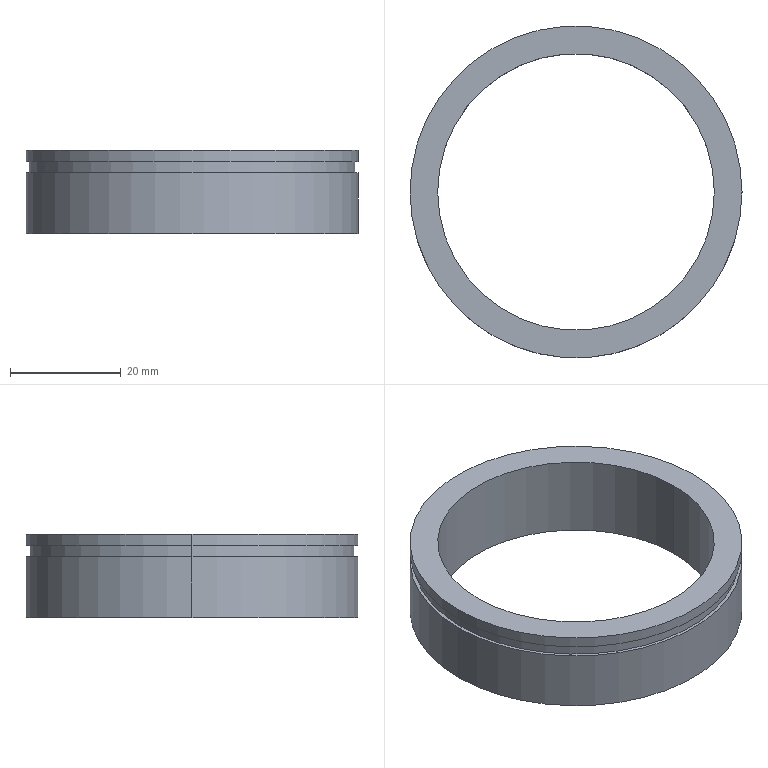Part | STEP file | 1 solid | 12 faces | box 60 x 60 x 15 mm | volume 12735 mm3 | cylinder 8 | plane 4 | commonest cylinder face diameters 60 x4 50 x2 58.8 x2
STEP:
#1=CARTESIAN_POINT('',(0.,0.,0.));
#2=DIRECTION('',(0.,0.,1.));
#3=DIRECTION('',(1.,0.,0.));
#4=AXIS2_PLACEMENT_3D('',#1,#2,#3);
#5=CARTESIAN_POINT('',(29.4,0.,11.));
#6=VERTEX_POINT('',#5);
#7=CARTESIAN_POINT('',(-29.4,0.,11.));
#8=VERTEX_POINT('',#7);
#9=CARTESIAN_POINT('',(0.,0.,11.));
#10=DIRECTION('',(0.,0.,1.));
#11=DIRECTION('',(1.,0.,0.));
#12=AXIS2_PLACEMENT_3D('',#9,#10,#11);
#13=CIRCLE('',#12,29.4);
#14=CARTESIAN_POINT('',(0.,0.,11.));
#15=DIRECTION('',(0.,0.,1.));
#16=DIRECTION('',(1.,0.,0.));
#17=AXIS2_PLACEMENT_3D('',#14,#15,#16);
#18=CYLINDRICAL_SURFACE('',#17,29.4);
#19=CARTESIAN_POINT('',(0.,0.));
#20=DIRECTION('',(1.,0.));
#21=VECTOR('',#20,1.);
#22=LINE('',#19,#21);
#23=(GEOMETRIC_REPRESENTATION_CONTEXT(2)PARAMETRIC_REPRESENTATION_CONTEXT()REPRESENTATION_CONTEXT('',''));
#24=DEFINITIONAL_REPRESENTATION('',(#22),#23);
#25=PCURVE('',#18,#24);
#26=CARTESIAN_POINT('',(0.,0.,11.));
#27=DIRECTION('',(0.,0.,1.));
#28=DIRECTION('',(1.,0.,0.));
#29=AXIS2_PLACEMENT_3D('',#26,#27,#28);
#30=PLANE('',#29);
#31=CARTESIAN_POINT('',(0.,0.));
#32=DIRECTION('',(1.,0.));
#33=AXIS2_PLACEMENT_2D('',#31,#32);
#34=CIRCLE('',#33,29.4);
#35=(GEOMETRIC_REPRESENTATION_CONTEXT(2)PARAMETRIC_REPRESENTATION_CONTEXT()REPRESENTATION_CONTEXT('',''));
#36=DEFINITIONAL_REPRESENTATION('',(#34),#35);
#37=PCURVE('',#30,#36);
#38=SURFACE_CURVE('',#13,(#25,#37),.PCURVE_S1.);
#39=EDGE_CURVE('',#6,#8,#38,.T.);
#40=ORIENTED_EDGE('',*,*,#39,.T.);
#41=CARTESIAN_POINT('',(-29.4,0.,13.));
#42=VERTEX_POINT('',#41);
#43=CARTESIAN_POINT('',(-29.4,0.,11.));
#44=DIRECTION('',(0.,0.,1.));
#45=VECTOR('',#44,1.);
#46=LINE('',#43,#45);
#47=CARTESIAN_POINT('',(3.142,0.));
#48=DIRECTION('',(0.,1.));
#49=VECTOR('',#48,1.);
#50=LINE('',#47,#49);
#51=(GEOMETRIC_REPRESENTATION_CONTEXT(2)PARAMETRIC_REPRESENTATION_CONTEXT()REPRESENTATION_CONTEXT('',''));
#52=DEFINITIONAL_REPRESENTATION('',(#50),#51);
#53=PCURVE('',#18,#52);
#54=CARTESIAN_POINT('',(0.,0.,11.));
#55=DIRECTION('',(0.,0.,1.));
#56=DIRECTION('',(1.,0.,0.));
#57=AXIS2_PLACEMENT_3D('',#54,#55,#56);
#58=CYLINDRICAL_SURFACE('',#57,29.4);
#59=CARTESIAN_POINT('',(3.142,0.));
#60=DIRECTION('',(0.,1.));
#61=VECTOR('',#60,1.);
#62=LINE('',#59,#61);
#63=(GEOMETRIC_REPRESENTATION_CONTEXT(2)PARAMETRIC_REPRESENTATION_CONTEXT()REPRESENTATION_CONTEXT('',''));
#64=DEFINITIONAL_REPRESENTATION('',(#62),#63);
#65=PCURVE('',#58,#64);
#66=SURFACE_CURVE('',#46,(#53,#65),.PCURVE_S1.);
#67=EDGE_CURVE('',#8,#42,#66,.T.);
#68=ORIENTED_EDGE('',*,*,#67,.T.);
#69=CARTESIAN_POINT('',(29.4,0.,13.));
#70=VERTEX_POINT('',#69);
#71=CARTESIAN_POINT('',(0.,0.,13.));
#72=DIRECTION('',(0.,0.,1.));
#73=DIRECTION('',(1.,0.,0.));
#74=AXIS2_PLACEMENT_3D('',#71,#72,#73);
#75=CIRCLE('',#74,29.4);
#76=CARTESIAN_POINT('',(0.,2.));
#77=DIRECTION('',(1.,0.));
#78=VECTOR('',#77,1.);
#79=LINE('',#76,#78);
#80=(GEOMETRIC_REPRESENTATION_CONTEXT(2)PARAMETRIC_REPRESENTATION_CONTEXT()REPRESENTATION_CONTEXT('',''));
#81=DEFINITIONAL_REPRESENTATION('',(#79),#80);
#82=PCURVE('',#18,#81);
#83=CARTESIAN_POINT('',(0.,0.,13.));
#84=DIRECTION('',(0.,0.,1.));
#85=DIRECTION('',(1.,0.,0.));
#86=AXIS2_PLACEMENT_3D('',#83,#84,#85);
#87=PLANE('',#86);
#88=CARTESIAN_POINT('',(0.,0.));
#89=DIRECTION('',(1.,0.));
#90=AXIS2_PLACEMENT_2D('',#88,#89);
#91=CIRCLE('',#90,29.4);
#92=(GEOMETRIC_REPRESENTATION_CONTEXT(2)PARAMETRIC_REPRESENTATION_CONTEXT()REPRESENTATION_CONTEXT('',''));
#93=DEFINITIONAL_REPRESENTATION('',(#91),#92);
#94=PCURVE('',#87,#93);
#95=SURFACE_CURVE('',#75,(#82,#94),.PCURVE_S1.);
#96=EDGE_CURVE('',#70,#42,#95,.T.);
#97=ORIENTED_EDGE('',*,*,#96,.F.);
#98=CARTESIAN_POINT('',(29.4,0.,11.));
#99=DIRECTION('',(0.,0.,1.));
#100=VECTOR('',#99,1.);
#101=LINE('',#98,#100);
#102=CARTESIAN_POINT('',(0.,0.));
#103=DIRECTION('',(0.,1.));
#104=VECTOR('',#103,1.);
#105=LINE('',#102,#104);
#106=(GEOMETRIC_REPRESENTATION_CONTEXT(2)PARAMETRIC_REPRESENTATION_CONTEXT()REPRESENTATION_CONTEXT('',''));
#107=DEFINITIONAL_REPRESENTATION('',(#105),#106);
#108=PCURVE('',#18,#107);
#109=CARTESIAN_POINT('',(6.283,0.));
#110=DIRECTION('',(0.,1.));
#111=VECTOR('',#110,1.);
#112=LINE('',#109,#111);
#113=(GEOMETRIC_REPRESENTATION_CONTEXT(2)PARAMETRIC_REPRESENTATION_CONTEXT()REPRESENTATION_CONTEXT('',''));
#114=DEFINITIONAL_REPRESENTATION('',(#112),#113);
#115=PCURVE('',#58,#114);
#116=SURFACE_CURVE('',#101,(#108,#115),.PCURVE_S1.);
#117=EDGE_CURVE('',#6,#70,#116,.T.);
#118=ORIENTED_EDGE('',*,*,#117,.F.);
#119=EDGE_LOOP('',(#40,#68,#97,#118));
#120=FACE_BOUND('',#119,.T.);
#121=ADVANCED_FACE('',(#120),#18,.T.);
#122=CARTESIAN_POINT('',(-25.,0.,15.));
#123=VERTEX_POINT('',#122);
#124=CARTESIAN_POINT('',(-25.,0.,0.));
#125=VERTEX_POINT('',#124);
#126=CARTESIAN_POINT('',(-25.,0.,15.));
#127=DIRECTION('',(0.,0.,-1.));
#128=VECTOR('',#127,1.);
#129=LINE('',#126,#128);
#130=CARTESIAN_POINT('',(0.,0.,15.));
#131=DIRECTION('',(0.,0.,-1.));
#132=DIRECTION('',(-1.,0.,0.));
#133=AXIS2_PLACEMENT_3D('',#130,#131,#132);
#134=CYLINDRICAL_SURFACE('',#133,25.);
#135=CARTESIAN_POINT('',(6.283,0.));
#136=DIRECTION('',(0.,1.));
#137=VECTOR('',#136,1.);
#138=LINE('',#135,#137);
#139=(GEOMETRIC_REPRESENTATION_CONTEXT(2)PARAMETRIC_REPRESENTATION_CONTEXT()REPRESENTATION_CONTEXT('',''));
#140=DEFINITIONAL_REPRESENTATION('',(#138),#139);
#141=PCURVE('',#134,#140);
#142=CARTESIAN_POINT('',(0.,0.,15.));
#143=DIRECTION('',(0.,0.,-1.));
#144=DIRECTION('',(-1.,0.,0.));
#145=AXIS2_PLACEMENT_3D('',#142,#143,#144);
#146=CYLINDRICAL_SURFACE('',#145,25.);
#147=CARTESIAN_POINT('',(0.,0.));
#148=DIRECTION('',(0.,1.));
#149=VECTOR('',#148,1.);
#150=LINE('',#147,#149);
#151=(GEOMETRIC_REPRESENTATION_CONTEXT(2)PARAMETRIC_REPRESENTATION_CONTEXT()REPRESENTATION_CONTEXT('',''));
#152=DEFINITIONAL_REPRESENTATION('',(#150),#151);
#153=PCURVE('',#146,#152);
#154=SURFACE_CURVE('',#129,(#141,#153),.PCURVE_S1.);
#155=EDGE_CURVE('',#123,#125,#154,.T.);
#156=ORIENTED_EDGE('',*,*,#155,.T.);
#157=CARTESIAN_POINT('',(25.,0.,0.));
#158=VERTEX_POINT('',#157);
#159=CARTESIAN_POINT('',(0.,0.,0.));
#160=DIRECTION('',(0.,0.,1.));
#161=DIRECTION('',(1.,0.,0.));
#162=AXIS2_PLACEMENT_3D('',#159,#160,#161);
#163=CIRCLE('',#162,25.);
#164=CARTESIAN_POINT('',(9.425,15.));
#165=DIRECTION('',(-1.,0.));
#166=VECTOR('',#165,1.);
#167=LINE('',#164,#166);
#168=(GEOMETRIC_REPRESENTATION_CONTEXT(2)PARAMETRIC_REPRESENTATION_CONTEXT()REPRESENTATION_CONTEXT('',''));
#169=DEFINITIONAL_REPRESENTATION('',(#167),#168);
#170=PCURVE('',#134,#169);
#171=CARTESIAN_POINT('',(0.,0.,0.));
#172=DIRECTION('',(0.,0.,1.));
#173=DIRECTION('',(1.,0.,0.));
#174=AXIS2_PLACEMENT_3D('',#171,#172,#173);
#175=PLANE('',#174);
#176=CARTESIAN_POINT('',(0.,0.));
#177=DIRECTION('',(1.,0.));
#178=AXIS2_PLACEMENT_2D('',#176,#177);
#179=CIRCLE('',#178,25.);
#180=(GEOMETRIC_REPRESENTATION_CONTEXT(2)PARAMETRIC_REPRESENTATION_CONTEXT()REPRESENTATION_CONTEXT('',''));
#181=DEFINITIONAL_REPRESENTATION('',(#179),#180);
#182=PCURVE('',#175,#181);
#183=SURFACE_CURVE('',#163,(#170,#182),.PCURVE_S1.);
#184=EDGE_CURVE('',#125,#158,#183,.T.);
#185=ORIENTED_EDGE('',*,*,#184,.T.);
#186=CARTESIAN_POINT('',(25.,0.,15.));
#187=VERTEX_POINT('',#186);
#188=CARTESIAN_POINT('',(25.,0.,15.));
#189=DIRECTION('',(0.,0.,-1.));
#190=VECTOR('',#189,1.);
#191=LINE('',#188,#190);
#192=CARTESIAN_POINT('',(3.142,0.));
#193=DIRECTION('',(0.,1.));
#194=VECTOR('',#193,1.);
#195=LINE('',#192,#194);
#196=(GEOMETRIC_REPRESENTATION_CONTEXT(2)PARAMETRIC_REPRESENTATION_CONTEXT()REPRESENTATION_CONTEXT('',''));
#197=DEFINITIONAL_REPRESENTATION('',(#195),#196);
#198=PCURVE('',#134,#197);
#199=CARTESIAN_POINT('',(3.142,0.));
#200=DIRECTION('',(0.,1.));
#201=VECTOR('',#200,1.);
#202=LINE('',#199,#201);
#203=(GEOMETRIC_REPRESENTATION_CONTEXT(2)PARAMETRIC_REPRESENTATION_CONTEXT()REPRESENTATION_CONTEXT('',''));
#204=DEFINITIONAL_REPRESENTATION('',(#202),#203);
#205=PCURVE('',#146,#204);
#206=SURFACE_CURVE('',#191,(#198,#205),.PCURVE_S1.);
#207=EDGE_CURVE('',#187,#158,#206,.T.);
#208=ORIENTED_EDGE('',*,*,#207,.F.);
#209=CARTESIAN_POINT('',(0.,0.,15.));
#210=DIRECTION('',(0.,0.,1.));
#211=DIRECTION('',(1.,0.,0.));
#212=AXIS2_PLACEMENT_3D('',#209,#210,#211);
#213=CIRCLE('',#212,25.);
#214=CARTESIAN_POINT('',(9.425,0.));
#215=DIRECTION('',(-1.,0.));
#216=VECTOR('',#215,1.);
#217=LINE('',#214,#216);
#218=(GEOMETRIC_REPRESENTATION_CONTEXT(2)PARAMETRIC_REPRESENTATION_CONTEXT()REPRESENTATION_CONTEXT('',''));
#219=DEFINITIONAL_REPRESENTATION('',(#217),#218);
#220=PCURVE('',#134,#219);
#221=CARTESIAN_POINT('',(0.,0.,15.));
#222=DIRECTION('',(0.,0.,1.));
#223=DIRECTION('',(1.,0.,0.));
#224=AXIS2_PLACEMENT_3D('',#221,#222,#223);
#225=PLANE('',#224);
#226=CARTESIAN_POINT('',(0.,0.));
#227=DIRECTION('',(1.,0.));
#228=AXIS2_PLACEMENT_2D('',#226,#227);
#229=CIRCLE('',#228,25.);
#230=(GEOMETRIC_REPRESENTATION_CONTEXT(2)PARAMETRIC_REPRESENTATION_CONTEXT()REPRESENTATION_CONTEXT('',''));
#231=DEFINITIONAL_REPRESENTATION('',(#229),#230);
#232=PCURVE('',#225,#231);
#233=SURFACE_CURVE('',#213,(#220,#232),.PCURVE_S1.);
#234=EDGE_CURVE('',#123,#187,#233,.T.);
#235=ORIENTED_EDGE('',*,*,#234,.F.);
#236=EDGE_LOOP('',(#156,#185,#208,#235));
#237=FACE_BOUND('',#236,.F.);
#238=ADVANCED_FACE('',(#237),#134,.F.);
#239=CARTESIAN_POINT('',(30.,0.,15.));
#240=VERTEX_POINT('',#239);
#241=CARTESIAN_POINT('',(-30.,0.,15.));
#242=VERTEX_POINT('',#241);
#243=CARTESIAN_POINT('',(0.,0.,15.));
#244=DIRECTION('',(0.,0.,1.));
#245=DIRECTION('',(1.,0.,0.));
#246=AXIS2_PLACEMENT_3D('',#243,#244,#245);
#247=CIRCLE('',#246,30.);
#248=CARTESIAN_POINT('',(0.,0.,15.));
#249=DIRECTION('',(0.,0.,-1.));
#250=DIRECTION('',(-1.,0.,0.));
#251=AXIS2_PLACEMENT_3D('',#248,#249,#250);
#252=CYLINDRICAL_SURFACE('',#251,30.);
#253=CARTESIAN_POINT('',(3.142,0.));
#254=DIRECTION('',(-1.,0.));
#255=VECTOR('',#254,1.);
#256=LINE('',#253,#255);
#257=(GEOMETRIC_REPRESENTATION_CONTEXT(2)PARAMETRIC_REPRESENTATION_CONTEXT()REPRESENTATION_CONTEXT('',''));
#258=DEFINITIONAL_REPRESENTATION('',(#256),#257);
#259=PCURVE('',#252,#258);
#260=CARTESIAN_POINT('',(0.,0.));
#261=DIRECTION('',(1.,0.));
#262=AXIS2_PLACEMENT_2D('',#260,#261);
#263=CIRCLE('',#262,30.);
#264=(GEOMETRIC_REPRESENTATION_CONTEXT(2)PARAMETRIC_REPRESENTATION_CONTEXT()REPRESENTATION_CONTEXT('',''));
#265=DEFINITIONAL_REPRESENTATION('',(#263),#264);
#266=PCURVE('',#225,#265);
#267=SURFACE_CURVE('',#247,(#259,#266),.PCURVE_S1.);
#268=EDGE_CURVE('',#240,#242,#267,.T.);
#269=ORIENTED_EDGE('',*,*,#268,.F.);
#270=CARTESIAN_POINT('',(30.,0.,13.));
#271=VERTEX_POINT('',#270);
#272=CARTESIAN_POINT('',(30.,0.,15.));
#273=DIRECTION('',(0.,0.,-1.));
#274=VECTOR('',#273,1.);
#275=LINE('',#272,#274);
#276=CARTESIAN_POINT('',(3.142,0.));
#277=DIRECTION('',(0.,1.));
#278=VECTOR('',#277,1.);
#279=LINE('',#276,#278);
#280=(GEOMETRIC_REPRESENTATION_CONTEXT(2)PARAMETRIC_REPRESENTATION_CONTEXT()REPRESENTATION_CONTEXT('',''));
#281=DEFINITIONAL_REPRESENTATION('',(#279),#280);
#282=PCURVE('',#252,#281);
#283=CARTESIAN_POINT('',(0.,0.,15.));
#284=DIRECTION('',(0.,0.,-1.));
#285=DIRECTION('',(-1.,0.,0.));
#286=AXIS2_PLACEMENT_3D('',#283,#284,#285);
#287=CYLINDRICAL_SURFACE('',#286,30.);
#288=CARTESIAN_POINT('',(3.142,0.));
#289=DIRECTION('',(0.,1.));
#290=VECTOR('',#289,1.);
#291=LINE('',#288,#290);
#292=(GEOMETRIC_REPRESENTATION_CONTEXT(2)PARAMETRIC_REPRESENTATION_CONTEXT()REPRESENTATION_CONTEXT('',''));
#293=DEFINITIONAL_REPRESENTATION('',(#291),#292);
#294=PCURVE('',#287,#293);
#295=SURFACE_CURVE('',#275,(#282,#294),.PCURVE_S1.);
#296=EDGE_CURVE('',#240,#271,#295,.T.);
#297=ORIENTED_EDGE('',*,*,#296,.T.);
#298=CARTESIAN_POINT('',(-30.,0.,13.));
#299=VERTEX_POINT('',#298);
#300=CARTESIAN_POINT('',(0.,0.,13.));
#301=DIRECTION('',(0.,0.,1.));
#302=DIRECTION('',(1.,0.,0.));
#303=AXIS2_PLACEMENT_3D('',#300,#301,#302);
#304=CIRCLE('',#303,30.);
#305=CARTESIAN_POINT('',(3.142,2.));
#306=DIRECTION('',(-1.,0.));
#307=VECTOR('',#306,1.);
#308=LINE('',#305,#307);
#309=(GEOMETRIC_REPRESENTATION_CONTEXT(2)PARAMETRIC_REPRESENTATION_CONTEXT()REPRESENTATION_CONTEXT('',''));
#310=DEFINITIONAL_REPRESENTATION('',(#308),#309);
#311=PCURVE('',#252,#310);
#312=CARTESIAN_POINT('',(0.,0.));
#313=DIRECTION('',(1.,0.));
#314=AXIS2_PLACEMENT_2D('',#312,#313);
#315=CIRCLE('',#314,30.);
#316=(GEOMETRIC_REPRESENTATION_CONTEXT(2)PARAMETRIC_REPRESENTATION_CONTEXT()REPRESENTATION_CONTEXT('',''));
#317=DEFINITIONAL_REPRESENTATION('',(#315),#316);
#318=PCURVE('',#87,#317);
#319=SURFACE_CURVE('',#304,(#311,#318),.PCURVE_S1.);
#320=EDGE_CURVE('',#271,#299,#319,.T.);
#321=ORIENTED_EDGE('',*,*,#320,.T.);
#322=CARTESIAN_POINT('',(-30.,0.,15.));
#323=DIRECTION('',(0.,0.,-1.));
#324=VECTOR('',#323,1.);
#325=LINE('',#322,#324);
#326=CARTESIAN_POINT('',(0.,0.));
#327=DIRECTION('',(0.,1.));
#328=VECTOR('',#327,1.);
#329=LINE('',#326,#328);
#330=(GEOMETRIC_REPRESENTATION_CONTEXT(2)PARAMETRIC_REPRESENTATION_CONTEXT()REPRESENTATION_CONTEXT('',''));
#331=DEFINITIONAL_REPRESENTATION('',(#329),#330);
#332=PCURVE('',#252,#331);
#333=CARTESIAN_POINT('',(6.283,0.));
#334=DIRECTION('',(0.,1.));
#335=VECTOR('',#334,1.);
#336=LINE('',#333,#335);
#337=(GEOMETRIC_REPRESENTATION_CONTEXT(2)PARAMETRIC_REPRESENTATION_CONTEXT()REPRESENTATION_CONTEXT('',''));
#338=DEFINITIONAL_REPRESENTATION('',(#336),#337);
#339=PCURVE('',#287,#338);
#340=SURFACE_CURVE('',#325,(#332,#339),.PCURVE_S1.);
#341=EDGE_CURVE('',#242,#299,#340,.T.);
#342=ORIENTED_EDGE('',*,*,#341,.F.);
#343=EDGE_LOOP('',(#269,#297,#321,#342));
#344=FACE_BOUND('',#343,.T.);
#345=ADVANCED_FACE('',(#344),#252,.T.);
#346=CARTESIAN_POINT('',(30.,0.,11.));
#347=VERTEX_POINT('',#346);
#348=CARTESIAN_POINT('',(-30.,0.,11.));
#349=VERTEX_POINT('',#348);
#350=CARTESIAN_POINT('',(0.,0.,11.));
#351=DIRECTION('',(0.,0.,1.));
#352=DIRECTION('',(1.,0.,0.));
#353=AXIS2_PLACEMENT_3D('',#350,#351,#352);
#354=CIRCLE('',#353,30.);
#355=CARTESIAN_POINT('',(0.,0.,15.));
#356=DIRECTION('',(0.,0.,-1.));
#357=DIRECTION('',(-1.,0.,0.));
#358=AXIS2_PLACEMENT_3D('',#355,#356,#357);
#359=CYLINDRICAL_SURFACE('',#358,30.);
#360=CARTESIAN_POINT('',(3.142,4.));
#361=DIRECTION('',(-1.,0.));
#362=VECTOR('',#361,1.);
#363=LINE('',#360,#362);
#364=(GEOMETRIC_REPRESENTATION_CONTEXT(2)PARAMETRIC_REPRESENTATION_CONTEXT()REPRESENTATION_CONTEXT('',''));
#365=DEFINITIONAL_REPRESENTATION('',(#363),#364);
#366=PCURVE('',#359,#365);
#367=CARTESIAN_POINT('',(0.,0.));
#368=DIRECTION('',(1.,0.));
#369=AXIS2_PLACEMENT_2D('',#367,#368);
#370=CIRCLE('',#369,30.);
#371=(GEOMETRIC_REPRESENTATION_CONTEXT(2)PARAMETRIC_REPRESENTATION_CONTEXT()REPRESENTATION_CONTEXT('',''));
#372=DEFINITIONAL_REPRESENTATION('',(#370),#371);
#373=PCURVE('',#30,#372);
#374=SURFACE_CURVE('',#354,(#366,#373),.PCURVE_S1.);
#375=EDGE_CURVE('',#347,#349,#374,.T.);
#376=ORIENTED_EDGE('',*,*,#375,.F.);
#377=CARTESIAN_POINT('',(30.,0.,0.));
#378=VERTEX_POINT('',#377);
#379=CARTESIAN_POINT('',(30.,0.,15.));
#380=DIRECTION('',(0.,0.,-1.));
#381=VECTOR('',#380,1.);
#382=LINE('',#379,#381);
#383=CARTESIAN_POINT('',(3.142,0.));
#384=DIRECTION('',(0.,1.));
#385=VECTOR('',#384,1.);
#386=LINE('',#383,#385);
#387=(GEOMETRIC_REPRESENTATION_CONTEXT(2)PARAMETRIC_REPRESENTATION_CONTEXT()REPRESENTATION_CONTEXT('',''));
#388=DEFINITIONAL_REPRESENTATION('',(#386),#387);
#389=PCURVE('',#359,#388);
#390=CARTESIAN_POINT('',(0.,0.,15.));
#391=DIRECTION('',(0.,0.,-1.));
#392=DIRECTION('',(-1.,0.,0.));
#393=AXIS2_PLACEMENT_3D('',#390,#391,#392);
#394=CYLINDRICAL_SURFACE('',#393,30.);
#395=CARTESIAN_POINT('',(3.142,0.));
#396=DIRECTION('',(0.,1.));
#397=VECTOR('',#396,1.);
#398=LINE('',#395,#397);
#399=(GEOMETRIC_REPRESENTATION_CONTEXT(2)PARAMETRIC_REPRESENTATION_CONTEXT()REPRESENTATION_CONTEXT('',''));
#400=DEFINITIONAL_REPRESENTATION('',(#398),#399);
#401=PCURVE('',#394,#400);
#402=SURFACE_CURVE('',#382,(#389,#401),.PCURVE_S1.);
#403=EDGE_CURVE('',#347,#378,#402,.T.);
#404=ORIENTED_EDGE('',*,*,#403,.T.);
#405=CARTESIAN_POINT('',(-30.,0.,0.));
#406=VERTEX_POINT('',#405);
#407=CARTESIAN_POINT('',(0.,0.,0.));
#408=DIRECTION('',(0.,0.,1.));
#409=DIRECTION('',(1.,0.,0.));
#410=AXIS2_PLACEMENT_3D('',#407,#408,#409);
#411=CIRCLE('',#410,30.);
#412=CARTESIAN_POINT('',(3.142,15.));
#413=DIRECTION('',(-1.,0.));
#414=VECTOR('',#413,1.);
#415=LINE('',#412,#414);
#416=(GEOMETRIC_REPRESENTATION_CONTEXT(2)PARAMETRIC_REPRESENTATION_CONTEXT()REPRESENTATION_CONTEXT('',''));
#417=DEFINITIONAL_REPRESENTATION('',(#415),#416);
#418=PCURVE('',#359,#417);
#419=CARTESIAN_POINT('',(0.,0.));
#420=DIRECTION('',(1.,0.));
#421=AXIS2_PLACEMENT_2D('',#419,#420);
#422=CIRCLE('',#421,30.);
#423=(GEOMETRIC_REPRESENTATION_CONTEXT(2)PARAMETRIC_REPRESENTATION_CONTEXT()REPRESENTATION_CONTEXT('',''));
#424=DEFINITIONAL_REPRESENTATION('',(#422),#423);
#425=PCURVE('',#175,#424);
#426=SURFACE_CURVE('',#411,(#418,#425),.PCURVE_S1.);
#427=EDGE_CURVE('',#378,#406,#426,.T.);
#428=ORIENTED_EDGE('',*,*,#427,.T.);
#429=CARTESIAN_POINT('',(-30.,0.,15.));
#430=DIRECTION('',(0.,0.,-1.));
#431=VECTOR('',#430,1.);
#432=LINE('',#429,#431);
#433=CARTESIAN_POINT('',(0.,0.));
#434=DIRECTION('',(0.,1.));
#435=VECTOR('',#434,1.);
#436=LINE('',#433,#435);
#437=(GEOMETRIC_REPRESENTATION_CONTEXT(2)PARAMETRIC_REPRESENTATION_CONTEXT()REPRESENTATION_CONTEXT('',''));
#438=DEFINITIONAL_REPRESENTATION('',(#436),#437);
#439=PCURVE('',#359,#438);
#440=CARTESIAN_POINT('',(6.283,0.));
#441=DIRECTION('',(0.,1.));
#442=VECTOR('',#441,1.);
#443=LINE('',#440,#442);
#444=(GEOMETRIC_REPRESENTATION_CONTEXT(2)PARAMETRIC_REPRESENTATION_CONTEXT()REPRESENTATION_CONTEXT('',''));
#445=DEFINITIONAL_REPRESENTATION('',(#443),#444);
#446=PCURVE('',#394,#445);
#447=SURFACE_CURVE('',#432,(#439,#446),.PCURVE_S1.);
#448=EDGE_CURVE('',#349,#406,#447,.T.);
#449=ORIENTED_EDGE('',*,*,#448,.F.);
#450=EDGE_LOOP('',(#376,#404,#428,#449));
#451=FACE_BOUND('',#450,.T.);
#452=ADVANCED_FACE('',(#451),#359,.T.);
#453=ORIENTED_EDGE('',*,*,#403,.F.);
#454=CARTESIAN_POINT('',(0.,0.,11.));
#455=DIRECTION('',(0.,0.,1.));
#456=DIRECTION('',(1.,0.,0.));
#457=AXIS2_PLACEMENT_3D('',#454,#455,#456);
#458=CIRCLE('',#457,30.);
#459=CARTESIAN_POINT('',(9.425,4.));
#460=DIRECTION('',(-1.,0.));
#461=VECTOR('',#460,1.);
#462=LINE('',#459,#461);
#463=(GEOMETRIC_REPRESENTATION_CONTEXT(2)PARAMETRIC_REPRESENTATION_CONTEXT()REPRESENTATION_CONTEXT('',''));
#464=DEFINITIONAL_REPRESENTATION('',(#462),#463);
#465=PCURVE('',#394,#464);
#466=CARTESIAN_POINT('',(0.,0.));
#467=DIRECTION('',(1.,0.));
#468=AXIS2_PLACEMENT_2D('',#466,#467);
#469=CIRCLE('',#468,30.);
#470=(GEOMETRIC_REPRESENTATION_CONTEXT(2)PARAMETRIC_REPRESENTATION_CONTEXT()REPRESENTATION_CONTEXT('',''));
#471=DEFINITIONAL_REPRESENTATION('',(#469),#470);
#472=PCURVE('',#30,#471);
#473=SURFACE_CURVE('',#458,(#465,#472),.PCURVE_S1.);
#474=EDGE_CURVE('',#349,#347,#473,.T.);
#475=ORIENTED_EDGE('',*,*,#474,.F.);
#476=ORIENTED_EDGE('',*,*,#448,.T.);
#477=CARTESIAN_POINT('',(0.,0.,0.));
#478=DIRECTION('',(0.,0.,1.));
#479=DIRECTION('',(1.,0.,0.));
#480=AXIS2_PLACEMENT_3D('',#477,#478,#479);
#481=CIRCLE('',#480,30.);
#482=CARTESIAN_POINT('',(9.425,15.));
#483=DIRECTION('',(-1.,0.));
#484=VECTOR('',#483,1.);
#485=LINE('',#482,#484);
#486=(GEOMETRIC_REPRESENTATION_CONTEXT(2)PARAMETRIC_REPRESENTATION_CONTEXT()REPRESENTATION_CONTEXT('',''));
#487=DEFINITIONAL_REPRESENTATION('',(#485),#486);
#488=PCURVE('',#394,#487);
#489=CARTESIAN_POINT('',(0.,0.));
#490=DIRECTION('',(1.,0.));
#491=AXIS2_PLACEMENT_2D('',#489,#490);
#492=CIRCLE('',#491,30.);
#493=(GEOMETRIC_REPRESENTATION_CONTEXT(2)PARAMETRIC_REPRESENTATION_CONTEXT()REPRESENTATION_CONTEXT('',''));
#494=DEFINITIONAL_REPRESENTATION('',(#492),#493);
#495=PCURVE('',#175,#494);
#496=SURFACE_CURVE('',#481,(#488,#495),.PCURVE_S1.);
#497=EDGE_CURVE('',#406,#378,#496,.T.);
#498=ORIENTED_EDGE('',*,*,#497,.T.);
#499=EDGE_LOOP('',(#453,#475,#476,#498));
#500=FACE_BOUND('',#499,.T.);
#501=ADVANCED_FACE('',(#500),#394,.T.);
#502=CARTESIAN_POINT('',(0.,0.,15.));
#503=DIRECTION('',(0.,0.,1.));
#504=DIRECTION('',(1.,0.,0.));
#505=AXIS2_PLACEMENT_3D('',#502,#503,#504);
#506=CIRCLE('',#505,30.);
#507=CARTESIAN_POINT('',(0.,0.));
#508=DIRECTION('',(1.,0.));
#509=AXIS2_PLACEMENT_2D('',#507,#508);
#510=CIRCLE('',#509,30.);
#511=(GEOMETRIC_REPRESENTATION_CONTEXT(2)PARAMETRIC_REPRESENTATION_CONTEXT()REPRESENTATION_CONTEXT('',''));
#512=DEFINITIONAL_REPRESENTATION('',(#510),#511);
#513=PCURVE('',#225,#512);
#514=CARTESIAN_POINT('',(9.425,0.));
#515=DIRECTION('',(-1.,0.));
#516=VECTOR('',#515,1.);
#517=LINE('',#514,#516);
#518=(GEOMETRIC_REPRESENTATION_CONTEXT(2)PARAMETRIC_REPRESENTATION_CONTEXT()REPRESENTATION_CONTEXT('',''));
#519=DEFINITIONAL_REPRESENTATION('',(#517),#518);
#520=PCURVE('',#287,#519);
#521=SURFACE_CURVE('',#506,(#513,#520),.PCURVE_S1.);
#522=EDGE_CURVE('',#242,#240,#521,.T.);
#523=ORIENTED_EDGE('',*,*,#522,.T.);
#524=ORIENTED_EDGE('',*,*,#268,.T.);
#525=EDGE_LOOP('',(#523,#524));
#526=FACE_BOUND('',#525,.T.);
#527=ORIENTED_EDGE('',*,*,#234,.F.);
#528=CARTESIAN_POINT('',(0.,0.,15.));
#529=DIRECTION('',(0.,0.,1.));
#530=DIRECTION('',(1.,0.,0.));
#531=AXIS2_PLACEMENT_3D('',#528,#529,#530);
#532=CIRCLE('',#531,25.);
#533=CARTESIAN_POINT('',(0.,0.));
#534=DIRECTION('',(1.,0.));
#535=AXIS2_PLACEMENT_2D('',#533,#534);
#536=CIRCLE('',#535,25.);
#537=(GEOMETRIC_REPRESENTATION_CONTEXT(2)PARAMETRIC_REPRESENTATION_CONTEXT()REPRESENTATION_CONTEXT('',''));
#538=DEFINITIONAL_REPRESENTATION('',(#536),#537);
#539=PCURVE('',#225,#538);
#540=CARTESIAN_POINT('',(3.142,0.));
#541=DIRECTION('',(-1.,0.));
#542=VECTOR('',#541,1.);
#543=LINE('',#540,#542);
#544=(GEOMETRIC_REPRESENTATION_CONTEXT(2)PARAMETRIC_REPRESENTATION_CONTEXT()REPRESENTATION_CONTEXT('',''));
#545=DEFINITIONAL_REPRESENTATION('',(#543),#544);
#546=PCURVE('',#146,#545);
#547=SURFACE_CURVE('',#532,(#539,#546),.PCURVE_S1.);
#548=EDGE_CURVE('',#187,#123,#547,.T.);
#549=ORIENTED_EDGE('',*,*,#548,.F.);
#550=EDGE_LOOP('',(#527,#549));
#551=FACE_BOUND('',#550,.T.);
#552=ADVANCED_FACE('',(#526,#551),#225,.T.);
#553=ORIENTED_EDGE('',*,*,#497,.F.);
#554=ORIENTED_EDGE('',*,*,#427,.F.);
#555=EDGE_LOOP('',(#553,#554));
#556=FACE_BOUND('',#555,.T.);
#557=ORIENTED_EDGE('',*,*,#184,.T.);
#558=CARTESIAN_POINT('',(0.,0.,0.));
#559=DIRECTION('',(0.,0.,1.));
#560=DIRECTION('',(1.,0.,0.));
#561=AXIS2_PLACEMENT_3D('',#558,#559,#560);
#562=CIRCLE('',#561,25.);
#563=CARTESIAN_POINT('',(0.,0.));
#564=DIRECTION('',(1.,0.));
#565=AXIS2_PLACEMENT_2D('',#563,#564);
#566=CIRCLE('',#565,25.);
#567=(GEOMETRIC_REPRESENTATION_CONTEXT(2)PARAMETRIC_REPRESENTATION_CONTEXT()REPRESENTATION_CONTEXT('',''));
#568=DEFINITIONAL_REPRESENTATION('',(#566),#567);
#569=PCURVE('',#175,#568);
#570=CARTESIAN_POINT('',(3.142,15.));
#571=DIRECTION('',(-1.,0.));
#572=VECTOR('',#571,1.);
#573=LINE('',#570,#572);
#574=(GEOMETRIC_REPRESENTATION_CONTEXT(2)PARAMETRIC_REPRESENTATION_CONTEXT()REPRESENTATION_CONTEXT('',''));
#575=DEFINITIONAL_REPRESENTATION('',(#573),#574);
#576=PCURVE('',#146,#575);
#577=SURFACE_CURVE('',#562,(#569,#576),.PCURVE_S1.);
#578=EDGE_CURVE('',#158,#125,#577,.T.);
#579=ORIENTED_EDGE('',*,*,#578,.T.);
#580=EDGE_LOOP('',(#557,#579));
#581=FACE_BOUND('',#580,.T.);
#582=ADVANCED_FACE('',(#556,#581),#175,.F.);
#583=ORIENTED_EDGE('',*,*,#296,.F.);
#584=ORIENTED_EDGE('',*,*,#522,.F.);
#585=ORIENTED_EDGE('',*,*,#341,.T.);
#586=CARTESIAN_POINT('',(0.,0.,13.));
#587=DIRECTION('',(0.,0.,1.));
#588=DIRECTION('',(1.,0.,0.));
#589=AXIS2_PLACEMENT_3D('',#586,#587,#588);
#590=CIRCLE('',#589,30.);
#591=CARTESIAN_POINT('',(9.425,2.));
#592=DIRECTION('',(-1.,0.));
#593=VECTOR('',#592,1.);
#594=LINE('',#591,#593);
#595=(GEOMETRIC_REPRESENTATION_CONTEXT(2)PARAMETRIC_REPRESENTATION_CONTEXT()REPRESENTATION_CONTEXT('',''));
#596=DEFINITIONAL_REPRESENTATION('',(#594),#595);
#597=PCURVE('',#287,#596);
#598=CARTESIAN_POINT('',(0.,0.));
#599=DIRECTION('',(1.,0.));
#600=AXIS2_PLACEMENT_2D('',#598,#599);
#601=CIRCLE('',#600,30.);
#602=(GEOMETRIC_REPRESENTATION_CONTEXT(2)PARAMETRIC_REPRESENTATION_CONTEXT()REPRESENTATION_CONTEXT('',''));
#603=DEFINITIONAL_REPRESENTATION('',(#601),#602);
#604=PCURVE('',#87,#603);
#605=SURFACE_CURVE('',#590,(#597,#604),.PCURVE_S1.);
#606=EDGE_CURVE('',#299,#271,#605,.T.);
#607=ORIENTED_EDGE('',*,*,#606,.T.);
#608=EDGE_LOOP('',(#583,#584,#585,#607));
#609=FACE_BOUND('',#608,.T.);
#610=ADVANCED_FACE('',(#609),#287,.T.);
#611=ORIENTED_EDGE('',*,*,#578,.T.);
#612=ORIENTED_EDGE('',*,*,#155,.F.);
#613=ORIENTED_EDGE('',*,*,#548,.F.);
#614=ORIENTED_EDGE('',*,*,#207,.T.);
#615=EDGE_LOOP('',(#611,#612,#613,#614));
#616=FACE_BOUND('',#615,.F.);
#617=ADVANCED_FACE('',(#616),#146,.F.);
#618=ORIENTED_EDGE('',*,*,#39,.F.);
#619=CARTESIAN_POINT('',(0.,0.,11.));
#620=DIRECTION('',(0.,0.,1.));
#621=DIRECTION('',(1.,0.,0.));
#622=AXIS2_PLACEMENT_3D('',#619,#620,#621);
#623=CIRCLE('',#622,29.4);
#624=CARTESIAN_POINT('',(0.,0.));
#625=DIRECTION('',(1.,0.));
#626=AXIS2_PLACEMENT_2D('',#624,#625);
#627=CIRCLE('',#626,29.4);
#628=(GEOMETRIC_REPRESENTATION_CONTEXT(2)PARAMETRIC_REPRESENTATION_CONTEXT()REPRESENTATION_CONTEXT('',''));
#629=DEFINITIONAL_REPRESENTATION('',(#627),#628);
#630=PCURVE('',#30,#629);
#631=CARTESIAN_POINT('',(0.,0.));
#632=DIRECTION('',(1.,0.));
#633=VECTOR('',#632,1.);
#634=LINE('',#631,#633);
#635=(GEOMETRIC_REPRESENTATION_CONTEXT(2)PARAMETRIC_REPRESENTATION_CONTEXT()REPRESENTATION_CONTEXT('',''));
#636=DEFINITIONAL_REPRESENTATION('',(#634),#635);
#637=PCURVE('',#58,#636);
#638=SURFACE_CURVE('',#623,(#630,#637),.PCURVE_S1.);
#639=EDGE_CURVE('',#8,#6,#638,.T.);
#640=ORIENTED_EDGE('',*,*,#639,.F.);
#641=EDGE_LOOP('',(#618,#640));
#642=FACE_BOUND('',#641,.T.);
#643=ORIENTED_EDGE('',*,*,#474,.T.);
#644=ORIENTED_EDGE('',*,*,#375,.T.);
#645=EDGE_LOOP('',(#643,#644));
#646=FACE_BOUND('',#645,.T.);
#647=ADVANCED_FACE('',(#642,#646),#30,.T.);
#648=ORIENTED_EDGE('',*,*,#96,.T.);
#649=CARTESIAN_POINT('',(0.,0.,13.));
#650=DIRECTION('',(0.,0.,1.));
#651=DIRECTION('',(1.,0.,0.));
#652=AXIS2_PLACEMENT_3D('',#649,#650,#651);
#653=CIRCLE('',#652,29.4);
#654=CARTESIAN_POINT('',(0.,0.));
#655=DIRECTION('',(1.,0.));
#656=AXIS2_PLACEMENT_2D('',#654,#655);
#657=CIRCLE('',#656,29.4);
#658=(GEOMETRIC_REPRESENTATION_CONTEXT(2)PARAMETRIC_REPRESENTATION_CONTEXT()REPRESENTATION_CONTEXT('',''));
#659=DEFINITIONAL_REPRESENTATION('',(#657),#658);
#660=PCURVE('',#87,#659);
#661=CARTESIAN_POINT('',(0.,2.));
#662=DIRECTION('',(1.,0.));
#663=VECTOR('',#662,1.);
#664=LINE('',#661,#663);
#665=(GEOMETRIC_REPRESENTATION_CONTEXT(2)PARAMETRIC_REPRESENTATION_CONTEXT()REPRESENTATION_CONTEXT('',''));
#666=DEFINITIONAL_REPRESENTATION('',(#664),#665);
#667=PCURVE('',#58,#666);
#668=SURFACE_CURVE('',#653,(#660,#667),.PCURVE_S1.);
#669=EDGE_CURVE('',#42,#70,#668,.T.);
#670=ORIENTED_EDGE('',*,*,#669,.T.);
#671=EDGE_LOOP('',(#648,#670));
#672=FACE_BOUND('',#671,.T.);
#673=ORIENTED_EDGE('',*,*,#606,.F.);
#674=ORIENTED_EDGE('',*,*,#320,.F.);
#675=EDGE_LOOP('',(#673,#674));
#676=FACE_BOUND('',#675,.T.);
#677=ADVANCED_FACE('',(#672,#676),#87,.F.);
#678=ORIENTED_EDGE('',*,*,#67,.F.);
#679=ORIENTED_EDGE('',*,*,#639,.T.);
#680=ORIENTED_EDGE('',*,*,#117,.T.);
#681=ORIENTED_EDGE('',*,*,#669,.F.);
#682=EDGE_LOOP('',(#678,#679,#680,#681));
#683=FACE_BOUND('',#682,.T.);
#684=ADVANCED_FACE('',(#683),#58,.T.);
#685=CLOSED_SHELL('',(#121,#238,#345,#452,#501,#552,#582,#610,#617,#647,#677,#684));
#686=MANIFOLD_SOLID_BREP('',#685);
#687=(LENGTH_UNIT()NAMED_UNIT(*)SI_UNIT(.MILLI.,.METRE.));
#688=UNCERTAINTY_MEASURE_WITH_UNIT(LENGTH_MEASURE(0.0000001),#687,'','');
#689=(NAMED_UNIT(*)PLANE_ANGLE_UNIT()SI_UNIT($,.RADIAN.));
#690=(NAMED_UNIT(*)SI_UNIT($,.STERADIAN.)SOLID_ANGLE_UNIT());
#691=(GEOMETRIC_REPRESENTATION_CONTEXT(3)GLOBAL_UNCERTAINTY_ASSIGNED_CONTEXT((#688))GLOBAL_UNIT_ASSIGNED_CONTEXT((#687,#689,#690))REPRESENTATION_CONTEXT('',''));
#692=ADVANCED_BREP_SHAPE_REPRESENTATION('',(#4,#686),#691);